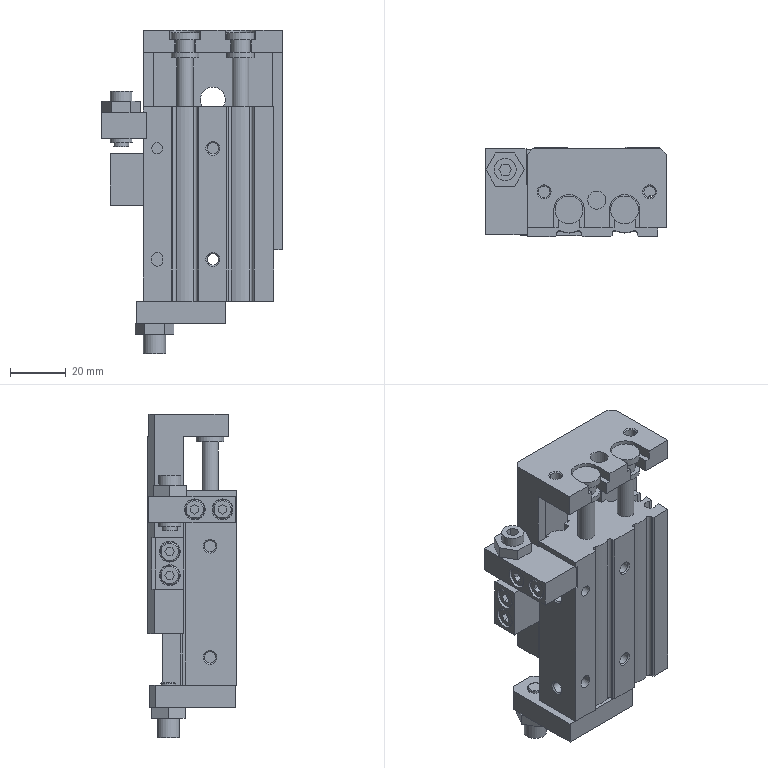Part | NX | 5 solids | 370 faces | box 65 x 32 x 116.533 mm | volume 116151 mm3 | plane 254 | cylinder 89 | cone 26 | spline 1 | commonest cylinder face diameters 3.242 x12 7.5 x10 4 x8 7 x8 2 x6 4.134 x6